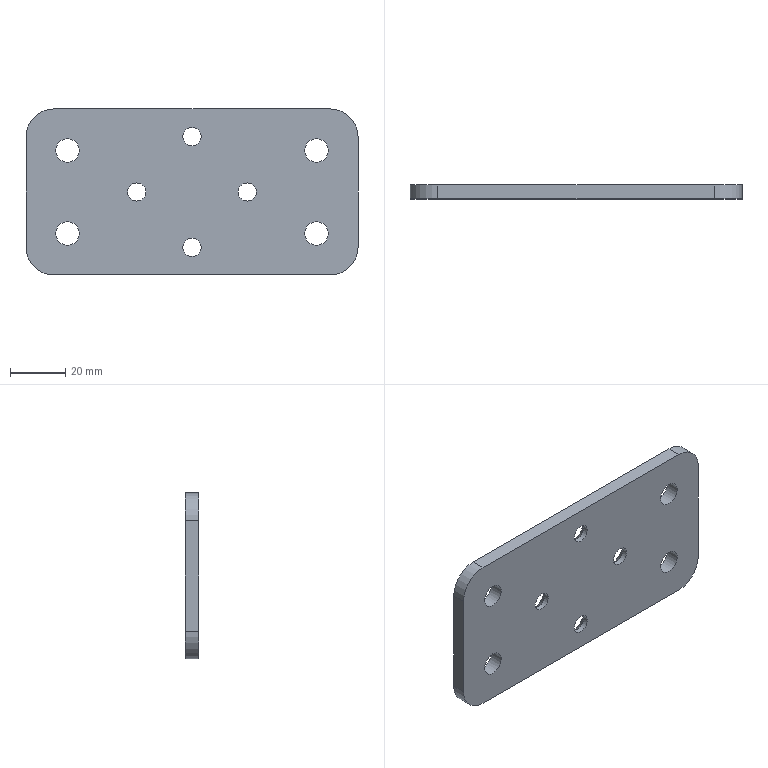Part | STEP file | JBJ-P-1011-10 | 1 solid | 22 faces | box 120 x 5 x 60 mm | volume 33228 mm3 | cylinder 12 | plane 6 | cone 4 | commonest cylinder face diameters 6.6 x4 8.5 x4 20 x4
STEP:
#1=CARTESIAN_POINT('',(60.,5.,56.4));
#2=VERTEX_POINT('',#1);
#3=CARTESIAN_POINT('',(60.,5.,50.));
#4=DIRECTION('',(0.,1.,0.));
#5=DIRECTION('',(0.,0.,1.));
#6=AXIS2_PLACEMENT_3D('',#3,#4,#5);
#7=CIRCLE('',#6,6.4);
#8=EDGE_CURVE('',#2,#2,#7,.T.);
#9=ORIENTED_EDGE('',*,*,#8,.F.);
#10=EDGE_LOOP('',(#9));
#11=FACE_BOUND('',#10,.T.);
#12=CARTESIAN_POINT('',(40.,5.,36.4));
#13=VERTEX_POINT('',#12);
#14=CARTESIAN_POINT('',(40.,5.,30.));
#15=DIRECTION('',(0.,1.,0.));
#16=DIRECTION('',(0.,0.,1.));
#17=AXIS2_PLACEMENT_3D('',#14,#15,#16);
#18=CIRCLE('',#17,6.4);
#19=EDGE_CURVE('',#13,#13,#18,.T.);
#20=ORIENTED_EDGE('',*,*,#19,.F.);
#21=EDGE_LOOP('',(#20));
#22=FACE_BOUND('',#21,.T.);
#23=CARTESIAN_POINT('',(80.,5.,36.4));
#24=VERTEX_POINT('',#23);
#25=CARTESIAN_POINT('',(80.,5.,30.));
#26=DIRECTION('',(0.,1.,0.));
#27=DIRECTION('',(0.,0.,1.));
#28=AXIS2_PLACEMENT_3D('',#25,#26,#27);
#29=CIRCLE('',#28,6.4);
#30=EDGE_CURVE('',#24,#24,#29,.T.);
#31=ORIENTED_EDGE('',*,*,#30,.F.);
#32=EDGE_LOOP('',(#31));
#33=FACE_BOUND('',#32,.T.);
#34=CARTESIAN_POINT('',(60.,5.,16.4));
#35=VERTEX_POINT('',#34);
#36=CARTESIAN_POINT('',(60.,5.,10.));
#37=DIRECTION('',(0.,1.,0.));
#38=DIRECTION('',(0.,0.,1.));
#39=AXIS2_PLACEMENT_3D('',#36,#37,#38);
#40=CIRCLE('',#39,6.4);
#41=EDGE_CURVE('',#35,#35,#40,.T.);
#42=ORIENTED_EDGE('',*,*,#41,.F.);
#43=EDGE_LOOP('',(#42));
#44=FACE_BOUND('',#43,.T.);
#45=CARTESIAN_POINT('',(105.,5.,49.25));
#46=VERTEX_POINT('',#45);
#47=CARTESIAN_POINT('',(105.,5.,45.));
#48=DIRECTION('',(0.,1.,0.));
#49=DIRECTION('',(0.,0.,1.));
#50=AXIS2_PLACEMENT_3D('',#47,#48,#49);
#51=CIRCLE('',#50,4.25);
#52=EDGE_CURVE('',#46,#46,#51,.T.);
#53=ORIENTED_EDGE('',*,*,#52,.F.);
#54=EDGE_LOOP('',(#53));
#55=FACE_BOUND('',#54,.T.);
#56=CARTESIAN_POINT('',(15.,5.,19.25));
#57=VERTEX_POINT('',#56);
#58=CARTESIAN_POINT('',(15.,5.,15.));
#59=DIRECTION('',(0.,1.,0.));
#60=DIRECTION('',(0.,0.,1.));
#61=AXIS2_PLACEMENT_3D('',#58,#59,#60);
#62=CIRCLE('',#61,4.25);
#63=EDGE_CURVE('',#57,#57,#62,.T.);
#64=ORIENTED_EDGE('',*,*,#63,.F.);
#65=EDGE_LOOP('',(#64));
#66=FACE_BOUND('',#65,.T.);
#67=CARTESIAN_POINT('',(0.,5.,10.));
#68=VERTEX_POINT('',#67);
#69=CARTESIAN_POINT('',(0.,5.,50.));
#70=VERTEX_POINT('',#69);
#71=CARTESIAN_POINT('',(0.,5.,0.));
#72=DIRECTION('',(0.,0.,1.));
#73=VECTOR('',#72,1000.);
#74=LINE('',#71,#73);
#75=EDGE_CURVE('',#68,#70,#74,.T.);
#76=ORIENTED_EDGE('',*,*,#75,.T.);
#77=CARTESIAN_POINT('',(10.,5.,60.));
#78=VERTEX_POINT('',#77);
#79=CARTESIAN_POINT('',(10.,5.,50.));
#80=DIRECTION('',(0.,1.,0.));
#81=DIRECTION('',(0.,0.,1.));
#82=AXIS2_PLACEMENT_3D('',#79,#80,#81);
#83=CIRCLE('',#82,10.);
#84=EDGE_CURVE('',#70,#78,#83,.T.);
#85=ORIENTED_EDGE('',*,*,#84,.T.);
#86=CARTESIAN_POINT('',(110.,5.,60.));
#87=VERTEX_POINT('',#86);
#88=CARTESIAN_POINT('',(0.,5.,60.));
#89=DIRECTION('',(1.,0.,0.));
#90=VECTOR('',#89,1000.);
#91=LINE('',#88,#90);
#92=EDGE_CURVE('',#78,#87,#91,.T.);
#93=ORIENTED_EDGE('',*,*,#92,.T.);
#94=CARTESIAN_POINT('',(120.,5.,50.));
#95=VERTEX_POINT('',#94);
#96=CARTESIAN_POINT('',(110.,5.,50.));
#97=DIRECTION('',(0.,1.,0.));
#98=DIRECTION('',(0.,0.,1.));
#99=AXIS2_PLACEMENT_3D('',#96,#97,#98);
#100=CIRCLE('',#99,10.);
#101=EDGE_CURVE('',#87,#95,#100,.T.);
#102=ORIENTED_EDGE('',*,*,#101,.T.);
#103=CARTESIAN_POINT('',(120.,5.,10.));
#104=VERTEX_POINT('',#103);
#105=CARTESIAN_POINT('',(120.,5.,0.));
#106=DIRECTION('',(0.,0.,-1.));
#107=VECTOR('',#106,1000.);
#108=LINE('',#105,#107);
#109=EDGE_CURVE('',#95,#104,#108,.T.);
#110=ORIENTED_EDGE('',*,*,#109,.T.);
#111=CARTESIAN_POINT('',(110.,5.,0.));
#112=VERTEX_POINT('',#111);
#113=CARTESIAN_POINT('',(110.,5.,10.));
#114=DIRECTION('',(0.,1.,0.));
#115=DIRECTION('',(0.,0.,1.));
#116=AXIS2_PLACEMENT_3D('',#113,#114,#115);
#117=CIRCLE('',#116,10.);
#118=EDGE_CURVE('',#104,#112,#117,.T.);
#119=ORIENTED_EDGE('',*,*,#118,.T.);
#120=CARTESIAN_POINT('',(10.,5.,0.));
#121=VERTEX_POINT('',#120);
#122=CARTESIAN_POINT('',(0.,5.,0.));
#123=DIRECTION('',(-1.,0.,0.));
#124=VECTOR('',#123,1000.);
#125=LINE('',#122,#124);
#126=EDGE_CURVE('',#112,#121,#125,.T.);
#127=ORIENTED_EDGE('',*,*,#126,.T.);
#128=CARTESIAN_POINT('',(10.,5.,10.));
#129=DIRECTION('',(0.,1.,0.));
#130=DIRECTION('',(0.,0.,1.));
#131=AXIS2_PLACEMENT_3D('',#128,#129,#130);
#132=CIRCLE('',#131,10.);
#133=EDGE_CURVE('',#121,#68,#132,.T.);
#134=ORIENTED_EDGE('',*,*,#133,.T.);
#135=EDGE_LOOP('',(#76,#85,#93,#102,#110,#119,#127,#134));
#136=FACE_OUTER_BOUND('',#135,.T.);
#137=CARTESIAN_POINT('',(15.,5.,40.75));
#138=VERTEX_POINT('',#137);
#139=CARTESIAN_POINT('',(15.,5.,45.));
#140=DIRECTION('',(0.,1.,0.));
#141=DIRECTION('',(0.,0.,-1.));
#142=AXIS2_PLACEMENT_3D('',#139,#140,#141);
#143=CIRCLE('',#142,4.25);
#144=EDGE_CURVE('',#138,#138,#143,.T.);
#145=ORIENTED_EDGE('',*,*,#144,.F.);
#146=EDGE_LOOP('',(#145));
#147=FACE_BOUND('',#146,.T.);
#148=CARTESIAN_POINT('',(105.,5.,10.75));
#149=VERTEX_POINT('',#148);
#150=CARTESIAN_POINT('',(105.,5.,15.));
#151=DIRECTION('',(0.,1.,0.));
#152=DIRECTION('',(0.,0.,-1.));
#153=AXIS2_PLACEMENT_3D('',#150,#151,#152);
#154=CIRCLE('',#153,4.25);
#155=EDGE_CURVE('',#149,#149,#154,.T.);
#156=ORIENTED_EDGE('',*,*,#155,.F.);
#157=EDGE_LOOP('',(#156));
#158=FACE_BOUND('',#157,.T.);
#159=CARTESIAN_POINT('',(0.,5.,0.));
#160=DIRECTION('',(0.,1.,0.));
#161=DIRECTION('',(0.,0.,1.));
#162=AXIS2_PLACEMENT_3D('',#159,#160,#161);
#163=PLANE('',#162);
#164=ADVANCED_FACE('',(#11,#22,#33,#44,#55,#66,#136,#147,#158),#163,.T.);
#165=CARTESIAN_POINT('',(60.,0.,53.3));
#166=VERTEX_POINT('',#165);
#167=CARTESIAN_POINT('',(60.,0.,50.));
#168=DIRECTION('',(0.,1.,0.));
#169=DIRECTION('',(0.,0.,1.));
#170=AXIS2_PLACEMENT_3D('',#167,#168,#169);
#171=CIRCLE('',#170,3.3);
#172=EDGE_CURVE('',#166,#166,#171,.T.);
#173=ORIENTED_EDGE('',*,*,#172,.T.);
#174=EDGE_LOOP('',(#173));
#175=FACE_BOUND('',#174,.T.);
#176=CARTESIAN_POINT('',(40.,0.,33.3));
#177=VERTEX_POINT('',#176);
#178=CARTESIAN_POINT('',(40.,0.,30.));
#179=DIRECTION('',(0.,1.,0.));
#180=DIRECTION('',(0.,0.,1.));
#181=AXIS2_PLACEMENT_3D('',#178,#179,#180);
#182=CIRCLE('',#181,3.3);
#183=EDGE_CURVE('',#177,#177,#182,.T.);
#184=ORIENTED_EDGE('',*,*,#183,.T.);
#185=EDGE_LOOP('',(#184));
#186=FACE_BOUND('',#185,.T.);
#187=CARTESIAN_POINT('',(80.,0.,33.3));
#188=VERTEX_POINT('',#187);
#189=CARTESIAN_POINT('',(80.,0.,30.));
#190=DIRECTION('',(0.,1.,0.));
#191=DIRECTION('',(0.,0.,1.));
#192=AXIS2_PLACEMENT_3D('',#189,#190,#191);
#193=CIRCLE('',#192,3.3);
#194=EDGE_CURVE('',#188,#188,#193,.T.);
#195=ORIENTED_EDGE('',*,*,#194,.T.);
#196=EDGE_LOOP('',(#195));
#197=FACE_BOUND('',#196,.T.);
#198=CARTESIAN_POINT('',(60.,0.,13.3));
#199=VERTEX_POINT('',#198);
#200=CARTESIAN_POINT('',(60.,0.,10.));
#201=DIRECTION('',(0.,1.,0.));
#202=DIRECTION('',(0.,0.,1.));
#203=AXIS2_PLACEMENT_3D('',#200,#201,#202);
#204=CIRCLE('',#203,3.3);
#205=EDGE_CURVE('',#199,#199,#204,.T.);
#206=ORIENTED_EDGE('',*,*,#205,.T.);
#207=EDGE_LOOP('',(#206));
#208=FACE_BOUND('',#207,.T.);
#209=CARTESIAN_POINT('',(10.,0.,60.));
#210=VERTEX_POINT('',#209);
#211=CARTESIAN_POINT('',(110.,0.,60.));
#212=VERTEX_POINT('',#211);
#213=CARTESIAN_POINT('',(0.,0.,60.));
#214=DIRECTION('',(1.,0.,0.));
#215=VECTOR('',#214,1000.);
#216=LINE('',#213,#215);
#217=EDGE_CURVE('',#210,#212,#216,.T.);
#218=ORIENTED_EDGE('',*,*,#217,.F.);
#219=CARTESIAN_POINT('',(0.,0.,50.));
#220=VERTEX_POINT('',#219);
#221=CARTESIAN_POINT('',(10.,0.,50.));
#222=DIRECTION('',(0.,-1.,0.));
#223=DIRECTION('',(0.,0.,1.));
#224=AXIS2_PLACEMENT_3D('',#221,#222,#223);
#225=CIRCLE('',#224,10.);
#226=EDGE_CURVE('',#210,#220,#225,.T.);
#227=ORIENTED_EDGE('',*,*,#226,.T.);
#228=CARTESIAN_POINT('',(0.,0.,10.));
#229=VERTEX_POINT('',#228);
#230=CARTESIAN_POINT('',(0.,0.,0.));
#231=DIRECTION('',(0.,0.,1.));
#232=VECTOR('',#231,1000.);
#233=LINE('',#230,#232);
#234=EDGE_CURVE('',#229,#220,#233,.T.);
#235=ORIENTED_EDGE('',*,*,#234,.F.);
#236=CARTESIAN_POINT('',(10.,0.,0.));
#237=VERTEX_POINT('',#236);
#238=CARTESIAN_POINT('',(10.,0.,10.));
#239=DIRECTION('',(0.,-1.,0.));
#240=DIRECTION('',(0.,0.,1.));
#241=AXIS2_PLACEMENT_3D('',#238,#239,#240);
#242=CIRCLE('',#241,10.);
#243=EDGE_CURVE('',#229,#237,#242,.T.);
#244=ORIENTED_EDGE('',*,*,#243,.T.);
#245=CARTESIAN_POINT('',(110.,0.,0.));
#246=VERTEX_POINT('',#245);
#247=CARTESIAN_POINT('',(0.,0.,0.));
#248=DIRECTION('',(-1.,0.,0.));
#249=VECTOR('',#248,1000.);
#250=LINE('',#247,#249);
#251=EDGE_CURVE('',#246,#237,#250,.T.);
#252=ORIENTED_EDGE('',*,*,#251,.F.);
#253=CARTESIAN_POINT('',(120.,0.,10.));
#254=VERTEX_POINT('',#253);
#255=CARTESIAN_POINT('',(110.,0.,10.));
#256=DIRECTION('',(0.,-1.,0.));
#257=DIRECTION('',(0.,0.,1.));
#258=AXIS2_PLACEMENT_3D('',#255,#256,#257);
#259=CIRCLE('',#258,10.);
#260=EDGE_CURVE('',#246,#254,#259,.T.);
#261=ORIENTED_EDGE('',*,*,#260,.T.);
#262=CARTESIAN_POINT('',(120.,0.,50.));
#263=VERTEX_POINT('',#262);
#264=CARTESIAN_POINT('',(120.,0.,0.));
#265=DIRECTION('',(0.,0.,-1.));
#266=VECTOR('',#265,1000.);
#267=LINE('',#264,#266);
#268=EDGE_CURVE('',#263,#254,#267,.T.);
#269=ORIENTED_EDGE('',*,*,#268,.F.);
#270=CARTESIAN_POINT('',(110.,0.,50.));
#271=DIRECTION('',(0.,-1.,0.));
#272=DIRECTION('',(0.,0.,1.));
#273=AXIS2_PLACEMENT_3D('',#270,#271,#272);
#274=CIRCLE('',#273,10.);
#275=EDGE_CURVE('',#263,#212,#274,.T.);
#276=ORIENTED_EDGE('',*,*,#275,.T.);
#277=EDGE_LOOP('',(#218,#227,#235,#244,#252,#261,#269,#276));
#278=FACE_OUTER_BOUND('',#277,.T.);
#279=CARTESIAN_POINT('',(15.,0.,19.25));
#280=VERTEX_POINT('',#279);
#281=CARTESIAN_POINT('',(15.,0.,15.));
#282=DIRECTION('',(0.,1.,0.));
#283=DIRECTION('',(0.,0.,1.));
#284=AXIS2_PLACEMENT_3D('',#281,#282,#283);
#285=CIRCLE('',#284,4.25);
#286=EDGE_CURVE('',#280,#280,#285,.T.);
#287=ORIENTED_EDGE('',*,*,#286,.T.);
#288=EDGE_LOOP('',(#287));
#289=FACE_BOUND('',#288,.T.);
#290=CARTESIAN_POINT('',(15.,0.,40.75));
#291=VERTEX_POINT('',#290);
#292=CARTESIAN_POINT('',(15.,0.,45.));
#293=DIRECTION('',(0.,1.,0.));
#294=DIRECTION('',(0.,0.,-1.));
#295=AXIS2_PLACEMENT_3D('',#292,#293,#294);
#296=CIRCLE('',#295,4.25);
#297=EDGE_CURVE('',#291,#291,#296,.T.);
#298=ORIENTED_EDGE('',*,*,#297,.T.);
#299=EDGE_LOOP('',(#298));
#300=FACE_BOUND('',#299,.T.);
#301=CARTESIAN_POINT('',(105.,0.,49.25));
#302=VERTEX_POINT('',#301);
#303=CARTESIAN_POINT('',(105.,0.,45.));
#304=DIRECTION('',(0.,1.,0.));
#305=DIRECTION('',(0.,0.,1.));
#306=AXIS2_PLACEMENT_3D('',#303,#304,#305);
#307=CIRCLE('',#306,4.25);
#308=EDGE_CURVE('',#302,#302,#307,.T.);
#309=ORIENTED_EDGE('',*,*,#308,.T.);
#310=EDGE_LOOP('',(#309));
#311=FACE_BOUND('',#310,.T.);
#312=CARTESIAN_POINT('',(105.,0.,10.75));
#313=VERTEX_POINT('',#312);
#314=CARTESIAN_POINT('',(105.,0.,15.));
#315=DIRECTION('',(0.,1.,0.));
#316=DIRECTION('',(0.,0.,-1.));
#317=AXIS2_PLACEMENT_3D('',#314,#315,#316);
#318=CIRCLE('',#317,4.25);
#319=EDGE_CURVE('',#313,#313,#318,.T.);
#320=ORIENTED_EDGE('',*,*,#319,.T.);
#321=EDGE_LOOP('',(#320));
#322=FACE_BOUND('',#321,.T.);
#323=CARTESIAN_POINT('',(0.,0.,0.));
#324=DIRECTION('',(0.,1.,0.));
#325=DIRECTION('',(0.,0.,1.));
#326=AXIS2_PLACEMENT_3D('',#323,#324,#325);
#327=PLANE('',#326);
#328=ADVANCED_FACE('',(#175,#186,#197,#208,#278,#289,#300,#311,#322),#327,.F.);
#329=ORIENTED_EDGE('',*,*,#234,.T.);
#330=CARTESIAN_POINT('',(0.,5.,50.));
#331=DIRECTION('',(0.,1.,0.));
#332=VECTOR('',#331,1000.);
#333=LINE('',#330,#332);
#334=EDGE_CURVE('',#220,#70,#333,.T.);
#335=ORIENTED_EDGE('',*,*,#334,.T.);
#336=ORIENTED_EDGE('',*,*,#75,.F.);
#337=CARTESIAN_POINT('',(0.,5.,10.));
#338=DIRECTION('',(0.,-1.,0.));
#339=VECTOR('',#338,1000.);
#340=LINE('',#337,#339);
#341=EDGE_CURVE('',#68,#229,#340,.T.);
#342=ORIENTED_EDGE('',*,*,#341,.T.);
#343=EDGE_LOOP('',(#329,#335,#336,#342));
#344=FACE_OUTER_BOUND('',#343,.T.);
#345=CARTESIAN_POINT('',(0.,5.,0.));
#346=DIRECTION('',(1.,0.,0.));
#347=DIRECTION('',(0.,0.,-1.));
#348=AXIS2_PLACEMENT_3D('',#345,#346,#347);
#349=PLANE('',#348);
#350=ADVANCED_FACE('',(#344),#349,.F.);
#351=ORIENTED_EDGE('',*,*,#92,.F.);
#352=CARTESIAN_POINT('',(10.,5.,60.));
#353=DIRECTION('',(0.,-1.,0.));
#354=VECTOR('',#353,1000.);
#355=LINE('',#352,#354);
#356=EDGE_CURVE('',#78,#210,#355,.T.);
#357=ORIENTED_EDGE('',*,*,#356,.T.);
#358=ORIENTED_EDGE('',*,*,#217,.T.);
#359=CARTESIAN_POINT('',(110.,5.,60.));
#360=DIRECTION('',(0.,1.,0.));
#361=VECTOR('',#360,1000.);
#362=LINE('',#359,#361);
#363=EDGE_CURVE('',#212,#87,#362,.T.);
#364=ORIENTED_EDGE('',*,*,#363,.T.);
#365=EDGE_LOOP('',(#351,#357,#358,#364));
#366=FACE_OUTER_BOUND('',#365,.T.);
#367=CARTESIAN_POINT('',(0.,5.,60.));
#368=DIRECTION('',(0.,0.,-1.));
#369=DIRECTION('',(-1.,0.,0.));
#370=AXIS2_PLACEMENT_3D('',#367,#368,#369);
#371=PLANE('',#370);
#372=ADVANCED_FACE('',(#366),#371,.F.);
#373=ORIENTED_EDGE('',*,*,#268,.T.);
#374=CARTESIAN_POINT('',(120.,5.,10.));
#375=DIRECTION('',(0.,1.,0.));
#376=VECTOR('',#375,1000.);
#377=LINE('',#374,#376);
#378=EDGE_CURVE('',#254,#104,#377,.T.);
#379=ORIENTED_EDGE('',*,*,#378,.T.);
#380=ORIENTED_EDGE('',*,*,#109,.F.);
#381=CARTESIAN_POINT('',(120.,5.,50.));
#382=DIRECTION('',(0.,-1.,0.));
#383=VECTOR('',#382,1000.);
#384=LINE('',#381,#383);
#385=EDGE_CURVE('',#95,#263,#384,.T.);
#386=ORIENTED_EDGE('',*,*,#385,.T.);
#387=EDGE_LOOP('',(#373,#379,#380,#386));
#388=FACE_OUTER_BOUND('',#387,.T.);
#389=CARTESIAN_POINT('',(120.,5.,0.));
#390=DIRECTION('',(-1.,0.,0.));
#391=DIRECTION('',(0.,0.,1.));
#392=AXIS2_PLACEMENT_3D('',#389,#390,#391);
#393=PLANE('',#392);
#394=ADVANCED_FACE('',(#388),#393,.F.);
#395=ORIENTED_EDGE('',*,*,#251,.T.);
#396=CARTESIAN_POINT('',(10.,5.,0.));
#397=DIRECTION('',(0.,1.,0.));
#398=VECTOR('',#397,1000.);
#399=LINE('',#396,#398);
#400=EDGE_CURVE('',#237,#121,#399,.T.);
#401=ORIENTED_EDGE('',*,*,#400,.T.);
#402=ORIENTED_EDGE('',*,*,#126,.F.);
#403=CARTESIAN_POINT('',(110.,5.,0.));
#404=DIRECTION('',(0.,-1.,0.));
#405=VECTOR('',#404,1000.);
#406=LINE('',#403,#405);
#407=EDGE_CURVE('',#112,#246,#406,.T.);
#408=ORIENTED_EDGE('',*,*,#407,.T.);
#409=EDGE_LOOP('',(#395,#401,#402,#408));
#410=FACE_OUTER_BOUND('',#409,.T.);
#411=CARTESIAN_POINT('',(0.,5.,0.));
#412=DIRECTION('',(0.,0.,1.));
#413=DIRECTION('',(1.,0.,0.));
#414=AXIS2_PLACEMENT_3D('',#411,#412,#413);
#415=PLANE('',#414);
#416=ADVANCED_FACE('',(#410),#415,.F.);
#417=ORIENTED_EDGE('',*,*,#63,.T.);
#418=EDGE_LOOP('',(#417));
#419=FACE_OUTER_BOUND('',#418,.T.);
#420=ORIENTED_EDGE('',*,*,#286,.F.);
#421=EDGE_LOOP('',(#420));
#422=FACE_OUTER_BOUND('',#421,.T.);
#423=CARTESIAN_POINT('',(15.,5.,15.));
#424=DIRECTION('',(0.,-1.,0.));
#425=DIRECTION('',(0.,0.,-1.));
#426=AXIS2_PLACEMENT_3D('',#423,#424,#425);
#427=CYLINDRICAL_SURFACE('',#426,4.25);
#428=ADVANCED_FACE('',(#419,#422),#427,.F.);
#429=ORIENTED_EDGE('',*,*,#144,.T.);
#430=EDGE_LOOP('',(#429));
#431=FACE_OUTER_BOUND('',#430,.T.);
#432=ORIENTED_EDGE('',*,*,#297,.F.);
#433=EDGE_LOOP('',(#432));
#434=FACE_OUTER_BOUND('',#433,.T.);
#435=CARTESIAN_POINT('',(15.,5.,45.));
#436=DIRECTION('',(0.,-1.,0.));
#437=DIRECTION('',(0.,0.,-1.));
#438=AXIS2_PLACEMENT_3D('',#435,#436,#437);
#439=CYLINDRICAL_SURFACE('',#438,4.25);
#440=ADVANCED_FACE('',(#431,#434),#439,.F.);
#441=ORIENTED_EDGE('',*,*,#52,.T.);
#442=EDGE_LOOP('',(#441));
#443=FACE_OUTER_BOUND('',#442,.T.);
#444=ORIENTED_EDGE('',*,*,#308,.F.);
#445=EDGE_LOOP('',(#444));
#446=FACE_OUTER_BOUND('',#445,.T.);
#447=CARTESIAN_POINT('',(105.,5.,45.));
#448=DIRECTION('',(0.,-1.,0.));
#449=DIRECTION('',(0.,0.,-1.));
#450=AXIS2_PLACEMENT_3D('',#447,#448,#449);
#451=CYLINDRICAL_SURFACE('',#450,4.25);
#452=ADVANCED_FACE('',(#443,#446),#451,.F.);
#453=ORIENTED_EDGE('',*,*,#155,.T.);
#454=EDGE_LOOP('',(#453));
#455=FACE_OUTER_BOUND('',#454,.T.);
#456=ORIENTED_EDGE('',*,*,#319,.F.);
#457=EDGE_LOOP('',(#456));
#458=FACE_OUTER_BOUND('',#457,.T.);
#459=CARTESIAN_POINT('',(105.,5.,15.));
#460=DIRECTION('',(0.,-1.,0.));
#461=DIRECTION('',(0.,0.,-1.));
#462=AXIS2_PLACEMENT_3D('',#459,#460,#461);
#463=CYLINDRICAL_SURFACE('',#462,4.25);
#464=ADVANCED_FACE('',(#455,#458),#463,.F.);
#465=ORIENTED_EDGE('',*,*,#84,.F.);
#466=ORIENTED_EDGE('',*,*,#334,.F.);
#467=ORIENTED_EDGE('',*,*,#226,.F.);
#468=ORIENTED_EDGE('',*,*,#356,.F.);
#469=EDGE_LOOP('',(#465,#466,#467,#468));
#470=FACE_OUTER_BOUND('',#469,.T.);
#471=CARTESIAN_POINT('',(10.,5.,50.));
#472=DIRECTION('',(0.,-1.,0.));
#473=DIRECTION('',(0.,0.,-1.));
#474=AXIS2_PLACEMENT_3D('',#471,#472,#473);
#475=CYLINDRICAL_SURFACE('',#474,10.);
#476=ADVANCED_FACE('',(#470),#475,.T.);
#477=ORIENTED_EDGE('',*,*,#133,.F.);
#478=ORIENTED_EDGE('',*,*,#400,.F.);
#479=ORIENTED_EDGE('',*,*,#243,.F.);
#480=ORIENTED_EDGE('',*,*,#341,.F.);
#481=EDGE_LOOP('',(#477,#478,#479,#480));
#482=FACE_OUTER_BOUND('',#481,.T.);
#483=CARTESIAN_POINT('',(10.,5.,10.));
#484=DIRECTION('',(0.,-1.,0.));
#485=DIRECTION('',(0.,0.,-1.));
#486=AXIS2_PLACEMENT_3D('',#483,#484,#485);
#487=CYLINDRICAL_SURFACE('',#486,10.);
#488=ADVANCED_FACE('',(#482),#487,.T.);
#489=ORIENTED_EDGE('',*,*,#118,.F.);
#490=ORIENTED_EDGE('',*,*,#378,.F.);
#491=ORIENTED_EDGE('',*,*,#260,.F.);
#492=ORIENTED_EDGE('',*,*,#407,.F.);
#493=EDGE_LOOP('',(#489,#490,#491,#492));
#494=FACE_OUTER_BOUND('',#493,.T.);
#495=CARTESIAN_POINT('',(110.,5.,10.));
#496=DIRECTION('',(0.,-1.,0.));
#497=DIRECTION('',(0.,0.,-1.));
#498=AXIS2_PLACEMENT_3D('',#495,#496,#497);
#499=CYLINDRICAL_SURFACE('',#498,10.);
#500=ADVANCED_FACE('',(#494),#499,.T.);
#501=ORIENTED_EDGE('',*,*,#101,.F.);
#502=ORIENTED_EDGE('',*,*,#363,.F.);
#503=ORIENTED_EDGE('',*,*,#275,.F.);
#504=ORIENTED_EDGE('',*,*,#385,.F.);
#505=EDGE_LOOP('',(#501,#502,#503,#504));
#506=FACE_OUTER_BOUND('',#505,.T.);
#507=CARTESIAN_POINT('',(110.,5.,50.));
#508=DIRECTION('',(0.,-1.,0.));
#509=DIRECTION('',(0.,0.,-1.));
#510=AXIS2_PLACEMENT_3D('',#507,#508,#509);
#511=CYLINDRICAL_SURFACE('',#510,10.);
#512=ADVANCED_FACE('',(#506),#511,.T.);
#513=CARTESIAN_POINT('',(60.,1.9,13.3));
#514=VERTEX_POINT('',#513);
#515=CARTESIAN_POINT('',(60.,1.9,10.));
#516=DIRECTION('',(0.,1.,0.));
#517=DIRECTION('',(0.,0.,1.));
#518=AXIS2_PLACEMENT_3D('',#515,#516,#517);
#519=CIRCLE('',#518,3.3);
#520=EDGE_CURVE('',#514,#514,#519,.T.);
#521=ORIENTED_EDGE('',*,*,#520,.T.);
#522=EDGE_LOOP('',(#521));
#523=FACE_OUTER_BOUND('',#522,.T.);
#524=ORIENTED_EDGE('',*,*,#205,.F.);
#525=EDGE_LOOP('',(#524));
#526=FACE_OUTER_BOUND('',#525,.T.);
#527=CARTESIAN_POINT('',(60.,5.,10.));
#528=DIRECTION('',(0.,1.,0.));
#529=DIRECTION('',(0.,0.,1.));
#530=AXIS2_PLACEMENT_3D('',#527,#528,#529);
#531=CYLINDRICAL_SURFACE('',#530,3.3);
#532=ADVANCED_FACE('',(#523,#526),#531,.F.);
#533=ORIENTED_EDGE('',*,*,#520,.F.);
#534=EDGE_LOOP('',(#533));
#535=FACE_BOUND('',#534,.T.);
#536=ORIENTED_EDGE('',*,*,#41,.T.);
#537=EDGE_LOOP('',(#536));
#538=FACE_OUTER_BOUND('',#537,.T.);
#539=CARTESIAN_POINT('',(60.,5.,10.));
#540=DIRECTION('',(0.,1.,0.));
#541=DIRECTION('',(0.,0.,1.));
#542=AXIS2_PLACEMENT_3D('',#539,#540,#541);
#543=CONICAL_SURFACE('',#542,6.4,0.7854);
#544=ADVANCED_FACE('',(#535,#538),#543,.F.);
#545=CARTESIAN_POINT('',(80.,1.9,33.3));
#546=VERTEX_POINT('',#545);
#547=CARTESIAN_POINT('',(80.,1.9,30.));
#548=DIRECTION('',(0.,1.,0.));
#549=DIRECTION('',(0.,0.,1.));
#550=AXIS2_PLACEMENT_3D('',#547,#548,#549);
#551=CIRCLE('',#550,3.3);
#552=EDGE_CURVE('',#546,#546,#551,.T.);
#553=ORIENTED_EDGE('',*,*,#552,.T.);
#554=EDGE_LOOP('',(#553));
#555=FACE_OUTER_BOUND('',#554,.T.);
#556=ORIENTED_EDGE('',*,*,#194,.F.);
#557=EDGE_LOOP('',(#556));
#558=FACE_OUTER_BOUND('',#557,.T.);
#559=CARTESIAN_POINT('',(80.,5.,30.));
#560=DIRECTION('',(0.,1.,0.));
#561=DIRECTION('',(0.,0.,1.));
#562=AXIS2_PLACEMENT_3D('',#559,#560,#561);
#563=CYLINDRICAL_SURFACE('',#562,3.3);
#564=ADVANCED_FACE('',(#555,#558),#563,.F.);
#565=ORIENTED_EDGE('',*,*,#552,.F.);
#566=EDGE_LOOP('',(#565));
#567=FACE_BOUND('',#566,.T.);
#568=ORIENTED_EDGE('',*,*,#30,.T.);
#569=EDGE_LOOP('',(#568));
#570=FACE_OUTER_BOUND('',#569,.T.);
#571=CARTESIAN_POINT('',(80.,5.,30.));
#572=DIRECTION('',(0.,1.,0.));
#573=DIRECTION('',(0.,0.,1.));
#574=AXIS2_PLACEMENT_3D('',#571,#572,#573);
#575=CONICAL_SURFACE('',#574,6.4,0.7854);
#576=ADVANCED_FACE('',(#567,#570),#575,.F.);
#577=CARTESIAN_POINT('',(40.,1.9,33.3));
#578=VERTEX_POINT('',#577);
#579=CARTESIAN_POINT('',(40.,1.9,30.));
#580=DIRECTION('',(0.,1.,0.));
#581=DIRECTION('',(0.,0.,1.));
#582=AXIS2_PLACEMENT_3D('',#579,#580,#581);
#583=CIRCLE('',#582,3.3);
#584=EDGE_CURVE('',#578,#578,#583,.T.);
#585=ORIENTED_EDGE('',*,*,#584,.T.);
#586=EDGE_LOOP('',(#585));
#587=FACE_OUTER_BOUND('',#586,.T.);
#588=ORIENTED_EDGE('',*,*,#183,.F.);
#589=EDGE_LOOP('',(#588));
#590=FACE_OUTER_BOUND('',#589,.T.);
#591=CARTESIAN_POINT('',(40.,5.,30.));
#592=DIRECTION('',(0.,1.,0.));
#593=DIRECTION('',(0.,0.,1.));
#594=AXIS2_PLACEMENT_3D('',#591,#592,#593);
#595=CYLINDRICAL_SURFACE('',#594,3.3);
#596=ADVANCED_FACE('',(#587,#590),#595,.F.);
#597=ORIENTED_EDGE('',*,*,#584,.F.);
#598=EDGE_LOOP('',(#597));
#599=FACE_BOUND('',#598,.T.);
#600=ORIENTED_EDGE('',*,*,#19,.T.);
#601=EDGE_LOOP('',(#600));
#602=FACE_OUTER_BOUND('',#601,.T.);
#603=CARTESIAN_POINT('',(40.,5.,30.));
#604=DIRECTION('',(0.,1.,0.));
#605=DIRECTION('',(0.,0.,1.));
#606=AXIS2_PLACEMENT_3D('',#603,#604,#605);
#607=CONICAL_SURFACE('',#606,6.4,0.7854);
#608=ADVANCED_FACE('',(#599,#602),#607,.F.);
#609=CARTESIAN_POINT('',(60.,1.9,53.3));
#610=VERTEX_POINT('',#609);
#611=CARTESIAN_POINT('',(60.,1.9,50.));
#612=DIRECTION('',(0.,1.,0.));
#613=DIRECTION('',(0.,0.,1.));
#614=AXIS2_PLACEMENT_3D('',#611,#612,#613);
#615=CIRCLE('',#614,3.3);
#616=EDGE_CURVE('',#610,#610,#615,.T.);
#617=ORIENTED_EDGE('',*,*,#616,.T.);
#618=EDGE_LOOP('',(#617));
#619=FACE_OUTER_BOUND('',#618,.T.);
#620=ORIENTED_EDGE('',*,*,#172,.F.);
#621=EDGE_LOOP('',(#620));
#622=FACE_OUTER_BOUND('',#621,.T.);
#623=CARTESIAN_POINT('',(60.,5.,50.));
#624=DIRECTION('',(0.,1.,0.));
#625=DIRECTION('',(0.,0.,1.));
#626=AXIS2_PLACEMENT_3D('',#623,#624,#625);
#627=CYLINDRICAL_SURFACE('',#626,3.3);
#628=ADVANCED_FACE('',(#619,#622),#627,.F.);
#629=ORIENTED_EDGE('',*,*,#616,.F.);
#630=EDGE_LOOP('',(#629));
#631=FACE_BOUND('',#630,.T.);
#632=ORIENTED_EDGE('',*,*,#8,.T.);
#633=EDGE_LOOP('',(#632));
#634=FACE_OUTER_BOUND('',#633,.T.);
#635=CARTESIAN_POINT('',(60.,5.,50.));
#636=DIRECTION('',(0.,1.,0.));
#637=DIRECTION('',(0.,0.,1.));
#638=AXIS2_PLACEMENT_3D('',#635,#636,#637);
#639=CONICAL_SURFACE('',#638,6.4,0.7854);
#640=ADVANCED_FACE('',(#631,#634),#639,.F.);
#641=CLOSED_SHELL('',(#164,#328,#350,#372,#394,#416,#428,#440,#452,#464,#476,#488,#500,#512,#532,#544,#564,#576,#596,#608,#628,#640));
#642=MANIFOLD_SOLID_BREP('',#641);
#643=CARTESIAN_POINT('',(0.,0.,0.));
#644=DIRECTION('',(0.,0.,1.));
#645=DIRECTION('',(1.,0.,0.));
#646=AXIS2_PLACEMENT_3D('',#643,#644,#645);
#647=(LENGTH_UNIT()NAMED_UNIT(*)SI_UNIT(.MILLI.,.METRE.));
#648=UNCERTAINTY_MEASURE_WITH_UNIT(LENGTH_MEASURE(0.00001),#647,'','');
#649=(NAMED_UNIT(*)PLANE_ANGLE_UNIT()SI_UNIT($,.RADIAN.));
#650=(NAMED_UNIT(*)SI_UNIT($,.STERADIAN.)SOLID_ANGLE_UNIT());
#651=(GEOMETRIC_REPRESENTATION_CONTEXT(3)GLOBAL_UNCERTAINTY_ASSIGNED_CONTEXT((#648))GLOBAL_UNIT_ASSIGNED_CONTEXT((#647,#649,#650))REPRESENTATION_CONTEXT('',''));
#652=ADVANCED_BREP_SHAPE_REPRESENTATION('',(#642,#646),#651);